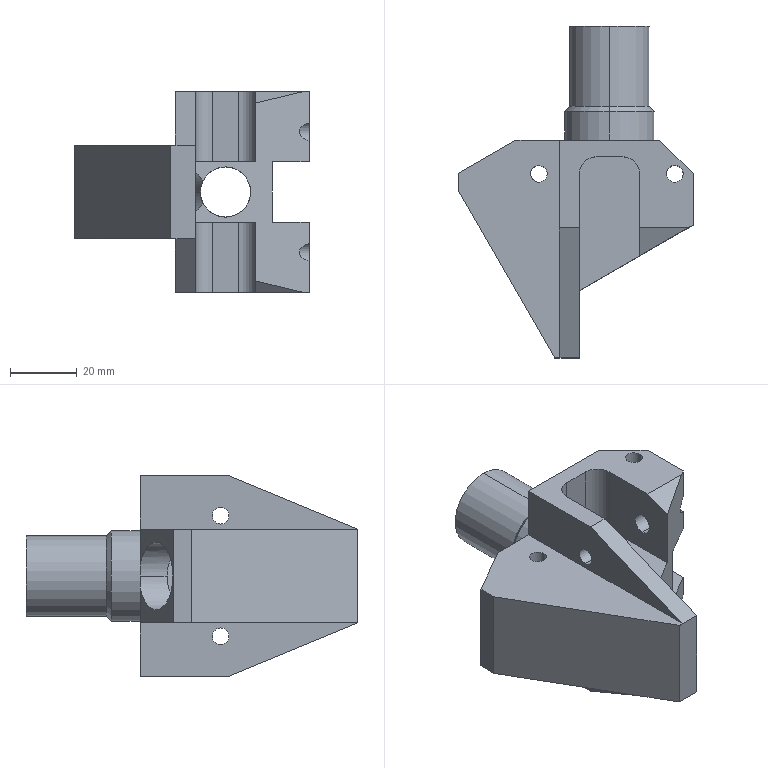Part | SolidWorks | features ICE 11, Chamfer 1, Extrusion 1, Fillet 1, MirrorPattern 1 | 1 solid | 63 faces | box 70 x 99.1 x 60 mm | volume 78724 mm3 | plane 33 | cylinder 28 | cone 2 | commonest cylinder face diameters 5 x10 6 x4 10 x4 13.5 x2 15 x2 20.2 x2